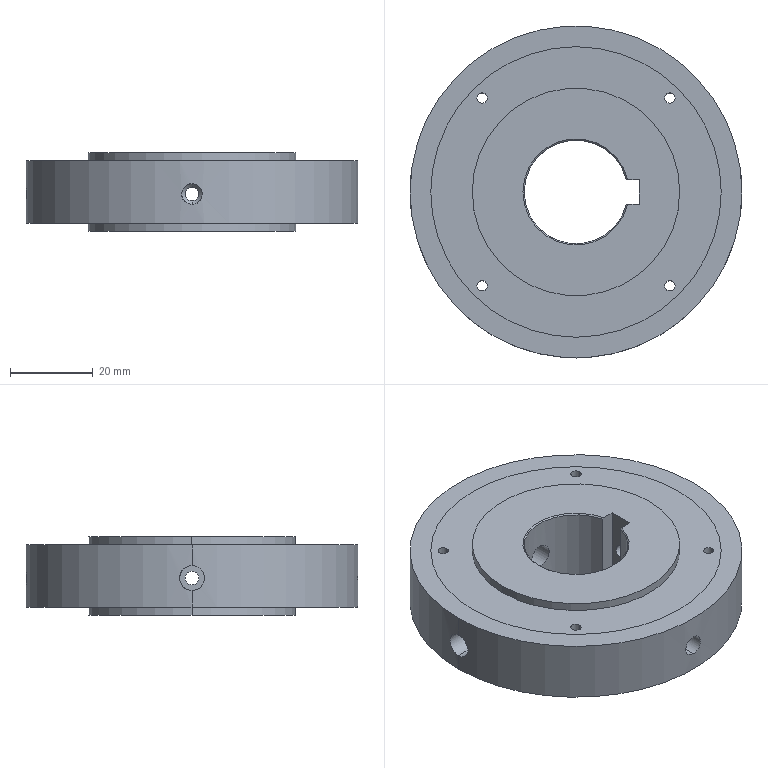Part | NX | features BREP 2 | 2 solids | 56 faces | box 80 x 80 x 19 mm | volume 70878 mm3 | cylinder 40 | plane 9 | cone 7 | commonest cylinder face diameters 2.5 x8 5 x8 6 x8 3.3 x4 50 x4 70 x4